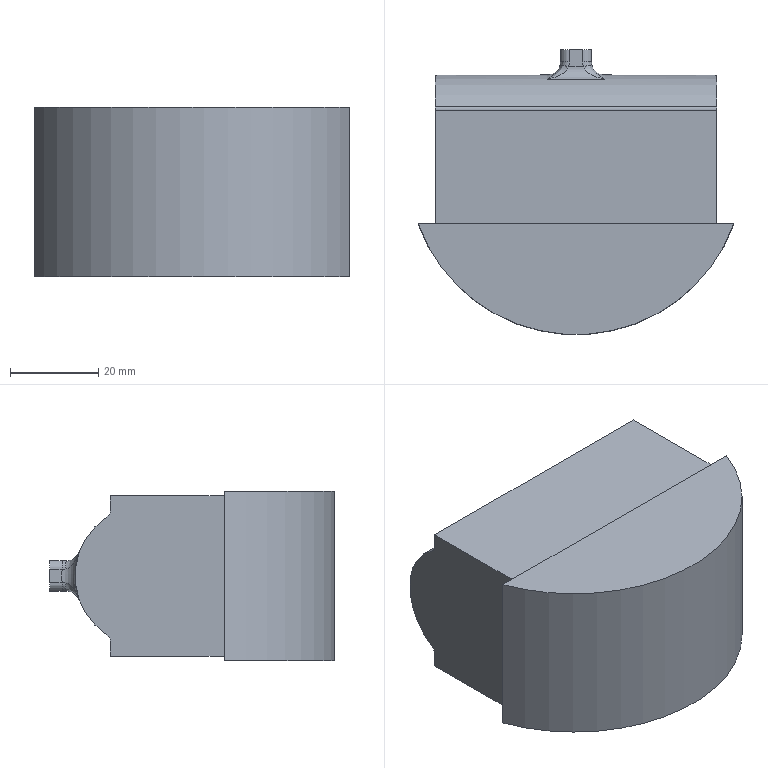Part | 1 solid | 34 faces | box 71.627 x 64.667 x 38.42 mm | volume 120668 mm3 | plane 14 | cylinder 10 | spline 8 | torus 2 | commonest cylinder face diameters 4 x4 3.6 x2 6 x2 32 x1 76.2 x1
STEP:
#1=CARTESIAN_POINT('',(-35.814,-13.,19.21));
#2=VERTEX_POINT('',#1);
#3=CARTESIAN_POINT('',(35.814,-13.,19.21));
#4=VERTEX_POINT('',#3);
#5=CARTESIAN_POINT('',(0.,0.,19.21));
#6=DIRECTION('',(0.,0.,1.));
#7=DIRECTION('',(1.,0.,0.));
#8=AXIS2_PLACEMENT_3D('',#5,#6,#7);
#9=CIRCLE('',#8,38.1);
#10=EDGE_CURVE('',#2,#4,#9,.T.);
#11=ORIENTED_EDGE('',*,*,#10,.F.);
#12=CARTESIAN_POINT('',(-35.814,-13.,-19.21));
#13=VERTEX_POINT('',#12);
#14=CARTESIAN_POINT('',(-35.814,-13.,-19.21));
#15=DIRECTION('',(0.,0.,1.));
#16=VECTOR('',#15,1000.);
#17=LINE('',#14,#16);
#18=EDGE_CURVE('',#2,#13,#17,.F.);
#19=ORIENTED_EDGE('',*,*,#18,.T.);
#20=CARTESIAN_POINT('',(35.814,-13.,-19.21));
#21=VERTEX_POINT('',#20);
#22=CARTESIAN_POINT('',(0.,0.,-19.21));
#23=DIRECTION('',(0.,0.,1.));
#24=DIRECTION('',(1.,0.,0.));
#25=AXIS2_PLACEMENT_3D('',#22,#23,#24);
#26=CIRCLE('',#25,38.1);
#27=EDGE_CURVE('',#13,#21,#26,.T.);
#28=ORIENTED_EDGE('',*,*,#27,.T.);
#29=CARTESIAN_POINT('',(35.814,-13.,-19.21));
#30=DIRECTION('',(0.,0.,1.));
#31=VECTOR('',#30,1000.);
#32=LINE('',#29,#31);
#33=EDGE_CURVE('',#21,#4,#32,.T.);
#34=ORIENTED_EDGE('',*,*,#33,.T.);
#35=EDGE_LOOP('',(#11,#19,#28,#34));
#36=FACE_BOUND('',#35,.T.);
#37=CARTESIAN_POINT('',(0.,0.,-19.21));
#38=DIRECTION('',(0.,0.,1.));
#39=DIRECTION('',(1.,0.,0.));
#40=AXIS2_PLACEMENT_3D('',#37,#38,#39);
#41=CYLINDRICAL_SURFACE('',#40,38.1);
#42=ADVANCED_FACE('',(#36),#41,.T.);
#43=CARTESIAN_POINT('',(0.,-13.,-19.21));
#44=DIRECTION('',(-1.,0.,0.));
#45=VECTOR('',#44,1000.);
#46=LINE('',#43,#45);
#47=EDGE_CURVE('',#21,#13,#46,.T.);
#48=ORIENTED_EDGE('',*,*,#47,.F.);
#49=ORIENTED_EDGE('',*,*,#27,.F.);
#50=EDGE_LOOP('',(#48,#49));
#51=FACE_BOUND('',#50,.T.);
#52=CARTESIAN_POINT('',(0.,0.,-19.21));
#53=DIRECTION('',(0.,0.,1.));
#54=DIRECTION('',(1.,0.,0.));
#55=AXIS2_PLACEMENT_3D('',#52,#53,#54);
#56=PLANE('',#55);
#57=ADVANCED_FACE('',(#51),#56,.F.);
#58=ORIENTED_EDGE('',*,*,#10,.T.);
#59=CARTESIAN_POINT('',(0.,-13.,19.21));
#60=DIRECTION('',(-1.,0.,0.));
#61=VECTOR('',#60,1000.);
#62=LINE('',#59,#61);
#63=EDGE_CURVE('',#4,#2,#62,.T.);
#64=ORIENTED_EDGE('',*,*,#63,.T.);
#65=EDGE_LOOP('',(#58,#64));
#66=FACE_BOUND('',#65,.T.);
#67=CARTESIAN_POINT('',(0.,0.,19.21));
#68=DIRECTION('',(0.,0.,1.));
#69=DIRECTION('',(1.,0.,0.));
#70=AXIS2_PLACEMENT_3D('',#67,#68,#69);
#71=PLANE('',#70);
#72=ADVANCED_FACE('',(#66),#71,.T.);
#73=CARTESIAN_POINT('',(31.91,-13.,18.207));
#74=VERTEX_POINT('',#73);
#75=CARTESIAN_POINT('',(31.91,-13.,-18.207));
#76=VERTEX_POINT('',#75);
#77=CARTESIAN_POINT('',(31.91,-13.,18.207));
#78=DIRECTION('',(0.,0.,-1.));
#79=VECTOR('',#78,1000.);
#80=LINE('',#77,#79);
#81=EDGE_CURVE('',#74,#76,#80,.T.);
#82=ORIENTED_EDGE('',*,*,#81,.F.);
#83=CARTESIAN_POINT('',(-31.91,-13.,18.207));
#84=VERTEX_POINT('',#83);
#85=CARTESIAN_POINT('',(-31.91,-13.,18.207));
#86=DIRECTION('',(1.,0.,0.));
#87=VECTOR('',#86,1000.);
#88=LINE('',#85,#87);
#89=EDGE_CURVE('',#84,#74,#88,.T.);
#90=ORIENTED_EDGE('',*,*,#89,.F.);
#91=CARTESIAN_POINT('',(-31.91,-13.,-18.207));
#92=VERTEX_POINT('',#91);
#93=CARTESIAN_POINT('',(-31.91,-13.,18.207));
#94=DIRECTION('',(0.,0.,1.));
#95=VECTOR('',#94,1000.);
#96=LINE('',#93,#95);
#97=EDGE_CURVE('',#92,#84,#96,.T.);
#98=ORIENTED_EDGE('',*,*,#97,.F.);
#99=CARTESIAN_POINT('',(-31.91,-13.,-18.207));
#100=DIRECTION('',(-1.,0.,0.));
#101=VECTOR('',#100,1000.);
#102=LINE('',#99,#101);
#103=EDGE_CURVE('',#76,#92,#102,.T.);
#104=ORIENTED_EDGE('',*,*,#103,.F.);
#105=EDGE_LOOP('',(#82,#90,#98,#104));
#106=FACE_BOUND('',#105,.T.);
#107=ORIENTED_EDGE('',*,*,#47,.T.);
#108=ORIENTED_EDGE('',*,*,#18,.F.);
#109=ORIENTED_EDGE('',*,*,#63,.F.);
#110=ORIENTED_EDGE('',*,*,#33,.F.);
#111=EDGE_LOOP('',(#107,#108,#109,#110));
#112=FACE_BOUND('',#111,.T.);
#113=CARTESIAN_POINT('',(0.,-13.,0.));
#114=DIRECTION('',(0.,1.,0.));
#115=DIRECTION('',(0.,0.,1.));
#116=AXIS2_PLACEMENT_3D('',#113,#114,#115);
#117=PLANE('',#116);
#118=ADVANCED_FACE('',(#106,#112),#117,.T.);
#119=CARTESIAN_POINT('',(31.91,12.817,-18.207));
#120=VERTEX_POINT('',#119);
#121=CARTESIAN_POINT('',(-31.91,12.817,-18.207));
#122=VERTEX_POINT('',#121);
#123=CARTESIAN_POINT('',(-31.91,12.817,-18.207));
#124=DIRECTION('',(-1.,0.,0.));
#125=VECTOR('',#124,1000.);
#126=LINE('',#123,#125);
#127=EDGE_CURVE('',#120,#122,#126,.T.);
#128=ORIENTED_EDGE('',*,*,#127,.F.);
#129=CARTESIAN_POINT('',(31.91,-13.,-18.207));
#130=DIRECTION('',(0.,1.,0.));
#131=VECTOR('',#130,1000.);
#132=LINE('',#129,#131);
#133=EDGE_CURVE('',#76,#120,#132,.T.);
#134=ORIENTED_EDGE('',*,*,#133,.F.);
#135=ORIENTED_EDGE('',*,*,#103,.T.);
#136=CARTESIAN_POINT('',(-31.91,-13.,-18.207));
#137=DIRECTION('',(0.,1.,0.));
#138=VECTOR('',#137,1000.);
#139=LINE('',#136,#138);
#140=EDGE_CURVE('',#92,#122,#139,.T.);
#141=ORIENTED_EDGE('',*,*,#140,.T.);
#142=EDGE_LOOP('',(#128,#134,#135,#141));
#143=FACE_BOUND('',#142,.T.);
#144=CARTESIAN_POINT('',(-31.91,-13.,-18.207));
#145=DIRECTION('',(0.,0.,-1.));
#146=DIRECTION('',(-1.,0.,0.));
#147=AXIS2_PLACEMENT_3D('',#144,#145,#146);
#148=PLANE('',#147);
#149=ADVANCED_FACE('',(#143),#148,.T.);
#150=CARTESIAN_POINT('',(31.91,12.817,-14.859));
#151=VERTEX_POINT('',#150);
#152=CARTESIAN_POINT('',(31.91,12.817,-13.856));
#153=DIRECTION('',(0.,0.,-1.));
#154=VECTOR('',#153,1000.);
#155=LINE('',#152,#154);
#156=EDGE_CURVE('',#151,#120,#155,.T.);
#157=ORIENTED_EDGE('',*,*,#156,.F.);
#158=CARTESIAN_POINT('',(31.91,13.626,-13.357));
#159=VERTEX_POINT('',#158);
#160=CARTESIAN_POINT('',(31.91,14.617,-14.859));
#161=DIRECTION('',(1.,0.,0.));
#162=DIRECTION('',(0.,0.,-1.));
#163=AXIS2_PLACEMENT_3D('',#160,#161,#162);
#164=CIRCLE('',#163,1.8);
#165=EDGE_CURVE('',#151,#159,#164,.F.);
#166=ORIENTED_EDGE('',*,*,#165,.T.);
#167=CARTESIAN_POINT('',(31.91,13.626,13.357));
#168=VERTEX_POINT('',#167);
#169=CARTESIAN_POINT('',(31.91,4.817,0.));
#170=DIRECTION('',(-1.,0.,0.));
#171=DIRECTION('',(0.,0.,-1.));
#172=AXIS2_PLACEMENT_3D('',#169,#170,#171);
#173=CIRCLE('',#172,16.);
#174=EDGE_CURVE('',#168,#159,#173,.T.);
#175=ORIENTED_EDGE('',*,*,#174,.F.);
#176=CARTESIAN_POINT('',(31.91,12.817,14.859));
#177=VERTEX_POINT('',#176);
#178=CARTESIAN_POINT('',(31.91,14.617,14.859));
#179=DIRECTION('',(1.,0.,0.));
#180=DIRECTION('',(0.,0.,-1.));
#181=AXIS2_PLACEMENT_3D('',#178,#179,#180);
#182=CIRCLE('',#181,1.8);
#183=EDGE_CURVE('',#168,#177,#182,.F.);
#184=ORIENTED_EDGE('',*,*,#183,.T.);
#185=CARTESIAN_POINT('',(31.91,12.817,18.207));
#186=VERTEX_POINT('',#185);
#187=CARTESIAN_POINT('',(31.91,12.817,20.785));
#188=DIRECTION('',(0.,0.,-1.));
#189=VECTOR('',#188,1000.);
#190=LINE('',#187,#189);
#191=EDGE_CURVE('',#186,#177,#190,.T.);
#192=ORIENTED_EDGE('',*,*,#191,.F.);
#193=CARTESIAN_POINT('',(31.91,-13.,18.207));
#194=DIRECTION('',(0.,1.,0.));
#195=VECTOR('',#194,1000.);
#196=LINE('',#193,#195);
#197=EDGE_CURVE('',#74,#186,#196,.T.);
#198=ORIENTED_EDGE('',*,*,#197,.F.);
#199=ORIENTED_EDGE('',*,*,#81,.T.);
#200=ORIENTED_EDGE('',*,*,#133,.T.);
#201=EDGE_LOOP('',(#157,#166,#175,#184,#192,#198,#199,#200));
#202=FACE_BOUND('',#201,.T.);
#203=CARTESIAN_POINT('',(31.91,-13.,18.207));
#204=DIRECTION('',(1.,0.,0.));
#205=DIRECTION('',(0.,0.,-1.));
#206=AXIS2_PLACEMENT_3D('',#203,#204,#205);
#207=PLANE('',#206);
#208=ADVANCED_FACE('',(#202),#207,.T.);
#209=CARTESIAN_POINT('',(-31.91,12.817,18.207));
#210=VERTEX_POINT('',#209);
#211=CARTESIAN_POINT('',(-31.91,12.817,18.207));
#212=DIRECTION('',(1.,0.,0.));
#213=VECTOR('',#212,1000.);
#214=LINE('',#211,#213);
#215=EDGE_CURVE('',#210,#186,#214,.T.);
#216=ORIENTED_EDGE('',*,*,#215,.F.);
#217=CARTESIAN_POINT('',(-31.91,-13.,18.207));
#218=DIRECTION('',(0.,1.,0.));
#219=VECTOR('',#218,1000.);
#220=LINE('',#217,#219);
#221=EDGE_CURVE('',#84,#210,#220,.T.);
#222=ORIENTED_EDGE('',*,*,#221,.F.);
#223=ORIENTED_EDGE('',*,*,#89,.T.);
#224=ORIENTED_EDGE('',*,*,#197,.T.);
#225=EDGE_LOOP('',(#216,#222,#223,#224));
#226=FACE_BOUND('',#225,.T.);
#227=CARTESIAN_POINT('',(-31.91,-13.,18.207));
#228=DIRECTION('',(0.,0.,1.));
#229=DIRECTION('',(1.,0.,0.));
#230=AXIS2_PLACEMENT_3D('',#227,#228,#229);
#231=PLANE('',#230);
#232=ADVANCED_FACE('',(#226),#231,.T.);
#233=CARTESIAN_POINT('',(-31.91,12.817,-14.859));
#234=VERTEX_POINT('',#233);
#235=CARTESIAN_POINT('',(-31.91,12.817,18.207));
#236=DIRECTION('',(0.,0.,1.));
#237=VECTOR('',#236,1000.);
#238=LINE('',#235,#237);
#239=EDGE_CURVE('',#122,#234,#238,.T.);
#240=ORIENTED_EDGE('',*,*,#239,.F.);
#241=ORIENTED_EDGE('',*,*,#140,.F.);
#242=ORIENTED_EDGE('',*,*,#97,.T.);
#243=ORIENTED_EDGE('',*,*,#221,.T.);
#244=CARTESIAN_POINT('',(-31.91,12.817,14.859));
#245=VERTEX_POINT('',#244);
#246=CARTESIAN_POINT('',(-31.91,12.817,18.207));
#247=DIRECTION('',(0.,0.,1.));
#248=VECTOR('',#247,1000.);
#249=LINE('',#246,#248);
#250=EDGE_CURVE('',#245,#210,#249,.T.);
#251=ORIENTED_EDGE('',*,*,#250,.F.);
#252=CARTESIAN_POINT('',(-31.91,13.626,13.357));
#253=VERTEX_POINT('',#252);
#254=CARTESIAN_POINT('',(-31.91,14.617,14.859));
#255=DIRECTION('',(-1.,0.,0.));
#256=DIRECTION('',(0.,0.,1.));
#257=AXIS2_PLACEMENT_3D('',#254,#255,#256);
#258=CIRCLE('',#257,1.8);
#259=EDGE_CURVE('',#245,#253,#258,.F.);
#260=ORIENTED_EDGE('',*,*,#259,.T.);
#261=CARTESIAN_POINT('',(-31.91,13.626,-13.357));
#262=VERTEX_POINT('',#261);
#263=CARTESIAN_POINT('',(-31.91,4.817,0.));
#264=DIRECTION('',(-1.,0.,0.));
#265=DIRECTION('',(0.,0.,1.));
#266=AXIS2_PLACEMENT_3D('',#263,#264,#265);
#267=CIRCLE('',#266,16.);
#268=EDGE_CURVE('',#262,#253,#267,.F.);
#269=ORIENTED_EDGE('',*,*,#268,.F.);
#270=CARTESIAN_POINT('',(-31.91,14.617,-14.859));
#271=DIRECTION('',(-1.,0.,0.));
#272=DIRECTION('',(0.,0.,1.));
#273=AXIS2_PLACEMENT_3D('',#270,#271,#272);
#274=CIRCLE('',#273,1.8);
#275=EDGE_CURVE('',#262,#234,#274,.F.);
#276=ORIENTED_EDGE('',*,*,#275,.T.);
#277=EDGE_LOOP('',(#240,#241,#242,#243,#251,#260,#269,#276));
#278=FACE_BOUND('',#277,.T.);
#279=CARTESIAN_POINT('',(-31.91,-13.,18.207));
#280=DIRECTION('',(-1.,0.,0.));
#281=DIRECTION('',(0.,0.,1.));
#282=AXIS2_PLACEMENT_3D('',#279,#280,#281);
#283=PLANE('',#282);
#284=ADVANCED_FACE('',(#278),#283,.T.);
#285=CARTESIAN_POINT('',(6.5,19.852,-5.474));
#286=VERTEX_POINT('',#285);
#287=CARTESIAN_POINT('',(6.5,19.852,5.474));
#288=VERTEX_POINT('',#287);
#289=CARTESIAN_POINT('',(6.5,4.817,0.));
#290=DIRECTION('',(1.,0.,0.));
#291=DIRECTION('',(0.,0.,-1.));
#292=AXIS2_PLACEMENT_3D('',#289,#290,#291);
#293=CIRCLE('',#292,16.);
#294=EDGE_CURVE('',#286,#288,#293,.T.);
#295=ORIENTED_EDGE('',*,*,#294,.T.);
#296=CARTESIAN_POINT('',(-6.5,19.852,5.474));
#297=VERTEX_POINT('',#296);
#298=CARTESIAN_POINT('',(-35.814,19.852,5.474));
#299=DIRECTION('',(1.,0.,0.));
#300=VECTOR('',#299,1000.);
#301=LINE('',#298,#300);
#302=EDGE_CURVE('',#288,#297,#301,.F.);
#303=ORIENTED_EDGE('',*,*,#302,.T.);
#304=CARTESIAN_POINT('',(-6.5,19.852,-5.474));
#305=VERTEX_POINT('',#304);
#306=CARTESIAN_POINT('',(-6.5,4.817,0.));
#307=DIRECTION('',(-1.,0.,0.));
#308=DIRECTION('',(0.,0.,1.));
#309=AXIS2_PLACEMENT_3D('',#306,#307,#308);
#310=CIRCLE('',#309,16.);
#311=EDGE_CURVE('',#297,#305,#310,.T.);
#312=ORIENTED_EDGE('',*,*,#311,.T.);
#313=CARTESIAN_POINT('',(-35.814,19.852,-5.474));
#314=DIRECTION('',(1.,0.,0.));
#315=VECTOR('',#314,1000.);
#316=LINE('',#313,#315);
#317=EDGE_CURVE('',#305,#286,#316,.T.);
#318=ORIENTED_EDGE('',*,*,#317,.T.);
#319=EDGE_LOOP('',(#295,#303,#312,#318));
#320=FACE_BOUND('',#319,.T.);
#321=ORIENTED_EDGE('',*,*,#268,.T.);
#322=CARTESIAN_POINT('',(-35.814,13.626,13.357));
#323=DIRECTION('',(1.,0.,0.));
#324=VECTOR('',#323,1000.);
#325=LINE('',#322,#324);
#326=EDGE_CURVE('',#253,#168,#325,.T.);
#327=ORIENTED_EDGE('',*,*,#326,.T.);
#328=ORIENTED_EDGE('',*,*,#174,.T.);
#329=CARTESIAN_POINT('',(-35.814,13.626,-13.357));
#330=DIRECTION('',(1.,0.,0.));
#331=VECTOR('',#330,1000.);
#332=LINE('',#329,#331);
#333=EDGE_CURVE('',#159,#262,#332,.F.);
#334=ORIENTED_EDGE('',*,*,#333,.T.);
#335=EDGE_LOOP('',(#321,#327,#328,#334));
#336=FACE_BOUND('',#335,.T.);
#337=CARTESIAN_POINT('',(-35.814,4.817,0.));
#338=DIRECTION('',(1.,0.,0.));
#339=DIRECTION('',(0.,0.,-1.));
#340=AXIS2_PLACEMENT_3D('',#337,#338,#339);
#341=CYLINDRICAL_SURFACE('',#340,16.);
#342=ADVANCED_FACE('',(#320,#336),#341,.T.);
#343=ORIENTED_EDGE('',*,*,#239,.T.);
#344=CARTESIAN_POINT('',(31.91,12.817,-14.859));
#345=DIRECTION('',(-1.,0.,0.));
#346=VECTOR('',#345,1000.);
#347=LINE('',#344,#346);
#348=EDGE_CURVE('',#234,#151,#347,.F.);
#349=ORIENTED_EDGE('',*,*,#348,.T.);
#350=ORIENTED_EDGE('',*,*,#156,.T.);
#351=ORIENTED_EDGE('',*,*,#127,.T.);
#352=EDGE_LOOP('',(#343,#349,#350,#351));
#353=FACE_BOUND('',#352,.T.);
#354=CARTESIAN_POINT('',(-35.814,12.817,-13.856));
#355=DIRECTION('',(0.,-1.,0.));
#356=DIRECTION('',(0.,0.,-1.));
#357=AXIS2_PLACEMENT_3D('',#354,#355,#356);
#358=PLANE('',#357);
#359=ADVANCED_FACE('',(#353),#358,.F.);
#360=ORIENTED_EDGE('',*,*,#191,.T.);
#361=CARTESIAN_POINT('',(-31.91,12.817,14.859));
#362=DIRECTION('',(-1.,0.,0.));
#363=VECTOR('',#362,1000.);
#364=LINE('',#361,#363);
#365=EDGE_CURVE('',#177,#245,#364,.T.);
#366=ORIENTED_EDGE('',*,*,#365,.T.);
#367=ORIENTED_EDGE('',*,*,#250,.T.);
#368=ORIENTED_EDGE('',*,*,#215,.T.);
#369=EDGE_LOOP('',(#360,#366,#367,#368));
#370=FACE_BOUND('',#369,.T.);
#371=CARTESIAN_POINT('',(-35.814,12.817,20.785));
#372=DIRECTION('',(0.,-1.,0.));
#373=DIRECTION('',(0.,0.,-1.));
#374=AXIS2_PLACEMENT_3D('',#371,#372,#373);
#375=PLANE('',#374);
#376=ADVANCED_FACE('',(#370),#375,.F.);
#377=ORIENTED_EDGE('',*,*,#259,.F.);
#378=ORIENTED_EDGE('',*,*,#365,.F.);
#379=ORIENTED_EDGE('',*,*,#183,.F.);
#380=ORIENTED_EDGE('',*,*,#326,.F.);
#381=EDGE_LOOP('',(#377,#378,#379,#380));
#382=FACE_BOUND('',#381,.T.);
#383=CARTESIAN_POINT('',(-35.814,14.617,14.859));
#384=DIRECTION('',(1.,0.,0.));
#385=DIRECTION('',(0.,0.,-1.));
#386=AXIS2_PLACEMENT_3D('',#383,#384,#385);
#387=CYLINDRICAL_SURFACE('',#386,1.8);
#388=ADVANCED_FACE('',(#382),#387,.F.);
#389=ORIENTED_EDGE('',*,*,#275,.F.);
#390=ORIENTED_EDGE('',*,*,#333,.F.);
#391=ORIENTED_EDGE('',*,*,#165,.F.);
#392=ORIENTED_EDGE('',*,*,#348,.F.);
#393=EDGE_LOOP('',(#389,#390,#391,#392));
#394=FACE_BOUND('',#393,.T.);
#395=CARTESIAN_POINT('',(-35.814,14.617,-14.859));
#396=DIRECTION('',(1.,0.,0.));
#397=DIRECTION('',(0.,0.,-1.));
#398=AXIS2_PLACEMENT_3D('',#395,#396,#397);
#399=CYLINDRICAL_SURFACE('',#398,1.8);
#400=ADVANCED_FACE('',(#394),#399,.F.);
#401=CARTESIAN_POINT('',(3.5,23.758,1.5));
#402=VERTEX_POINT('',#401);
#403=CARTESIAN_POINT('',(3.5,23.758,-1.5));
#404=VERTEX_POINT('',#403);
#405=CARTESIAN_POINT('',(3.5,4.817,0.));
#406=DIRECTION('',(1.,0.,0.));
#407=DIRECTION('',(0.,0.,-1.));
#408=AXIS2_PLACEMENT_3D('',#405,#406,#407);
#409=CIRCLE('',#408,19.);
#410=EDGE_CURVE('',#402,#404,#409,.F.);
#411=ORIENTED_EDGE('',*,*,#410,.T.);
#412=CARTESIAN_POINT('',(3.5,26.567,-1.5));
#413=VERTEX_POINT('',#412);
#414=CARTESIAN_POINT('',(3.5,16.924,-1.5));
#415=DIRECTION('',(0.,1.,0.));
#416=VECTOR('',#415,1000.);
#417=LINE('',#414,#416);
#418=EDGE_CURVE('',#404,#413,#417,.T.);
#419=ORIENTED_EDGE('',*,*,#418,.T.);
#420=CARTESIAN_POINT('',(3.5,26.567,1.5));
#421=VERTEX_POINT('',#420);
#422=CARTESIAN_POINT('',(3.5,26.567,-3.5));
#423=DIRECTION('',(0.,0.,-1.));
#424=VECTOR('',#423,1000.);
#425=LINE('',#422,#424);
#426=EDGE_CURVE('',#421,#413,#425,.T.);
#427=ORIENTED_EDGE('',*,*,#426,.F.);
#428=CARTESIAN_POINT('',(3.5,16.924,1.5));
#429=DIRECTION('',(0.,1.,0.));
#430=VECTOR('',#429,1000.);
#431=LINE('',#428,#430);
#432=EDGE_CURVE('',#421,#402,#431,.F.);
#433=ORIENTED_EDGE('',*,*,#432,.T.);
#434=EDGE_LOOP('',(#411,#419,#427,#433));
#435=FACE_BOUND('',#434,.T.);
#436=CARTESIAN_POINT('',(3.5,16.924,-3.5));
#437=DIRECTION('',(1.,0.,0.));
#438=DIRECTION('',(0.,0.,-1.));
#439=AXIS2_PLACEMENT_3D('',#436,#437,#438);
#440=PLANE('',#439);
#441=ADVANCED_FACE('',(#435),#440,.T.);
#442=CARTESIAN_POINT('',(-1.619,22.671,3.5));
#443=VERTEX_POINT('',#442);
#444=CARTESIAN_POINT('',(1.619,22.671,3.5));
#445=VERTEX_POINT('',#444);
#446=CARTESIAN_POINT('',(-3.5,22.671,3.5));
#447=DIRECTION('',(1.,0.,0.));
#448=VECTOR('',#447,1000.);
#449=LINE('',#446,#448);
#450=EDGE_CURVE('',#443,#445,#449,.T.);
#451=ORIENTED_EDGE('',*,*,#450,.T.);
#452=CARTESIAN_POINT('',(1.5,23.758,3.5));
#453=VERTEX_POINT('',#452);
#454=CARTESIAN_POINT('',(1.619,22.671,3.5));
#455=CARTESIAN_POINT('',(1.54,23.029,3.5));
#456=CARTESIAN_POINT('',(1.5,23.391,3.5));
#457=CARTESIAN_POINT('',(1.5,23.758,3.5));
#458=B_SPLINE_CURVE_WITH_KNOTS('',3,(#454,#455,#456,#457),.UNSPECIFIED.,.F.,.F.,(4,4),(0.,0.001094),.UNSPECIFIED.);
#459=EDGE_CURVE('',#445,#453,#458,.T.);
#460=ORIENTED_EDGE('',*,*,#459,.T.);
#461=CARTESIAN_POINT('',(1.5,26.567,3.5));
#462=VERTEX_POINT('',#461);
#463=CARTESIAN_POINT('',(1.5,16.924,3.5));
#464=DIRECTION('',(0.,1.,0.));
#465=VECTOR('',#464,1000.);
#466=LINE('',#463,#465);
#467=EDGE_CURVE('',#453,#462,#466,.T.);
#468=ORIENTED_EDGE('',*,*,#467,.T.);
#469=CARTESIAN_POINT('',(-1.5,26.567,3.5));
#470=VERTEX_POINT('',#469);
#471=CARTESIAN_POINT('',(-3.5,26.567,3.5));
#472=DIRECTION('',(1.,0.,0.));
#473=VECTOR('',#472,1000.);
#474=LINE('',#471,#473);
#475=EDGE_CURVE('',#470,#462,#474,.T.);
#476=ORIENTED_EDGE('',*,*,#475,.F.);
#477=CARTESIAN_POINT('',(-1.5,23.758,3.5));
#478=VERTEX_POINT('',#477);
#479=CARTESIAN_POINT('',(-1.5,16.924,3.5));
#480=DIRECTION('',(0.,1.,0.));
#481=VECTOR('',#480,1000.);
#482=LINE('',#479,#481);
#483=EDGE_CURVE('',#470,#478,#482,.F.);
#484=ORIENTED_EDGE('',*,*,#483,.T.);
#485=CARTESIAN_POINT('',(-1.5,23.758,3.5));
#486=CARTESIAN_POINT('',(-1.5,23.391,3.5));
#487=CARTESIAN_POINT('',(-1.54,23.029,3.5));
#488=CARTESIAN_POINT('',(-1.619,22.671,3.5));
#489=B_SPLINE_CURVE_WITH_KNOTS('',3,(#485,#486,#487,#488),.UNSPECIFIED.,.F.,.F.,(4,4),(0.,0.001094),.UNSPECIFIED.);
#490=EDGE_CURVE('',#478,#443,#489,.T.);
#491=ORIENTED_EDGE('',*,*,#490,.T.);
#492=EDGE_LOOP('',(#451,#460,#468,#476,#484,#491));
#493=FACE_BOUND('',#492,.T.);
#494=CARTESIAN_POINT('',(-3.5,16.924,3.5));
#495=DIRECTION('',(0.,0.,1.));
#496=DIRECTION('',(1.,0.,0.));
#497=AXIS2_PLACEMENT_3D('',#494,#495,#496);
#498=PLANE('',#497);
#499=ADVANCED_FACE('',(#493),#498,.T.);
#500=CARTESIAN_POINT('',(-3.5,26.567,-1.5));
#501=VERTEX_POINT('',#500);
#502=CARTESIAN_POINT('',(-3.5,26.567,1.5));
#503=VERTEX_POINT('',#502);
#504=CARTESIAN_POINT('',(-3.5,26.567,-3.5));
#505=DIRECTION('',(0.,0.,1.));
#506=VECTOR('',#505,1000.);
#507=LINE('',#504,#506);
#508=EDGE_CURVE('',#501,#503,#507,.T.);
#509=ORIENTED_EDGE('',*,*,#508,.F.);
#510=CARTESIAN_POINT('',(-3.5,23.758,-1.5));
#511=VERTEX_POINT('',#510);
#512=CARTESIAN_POINT('',(-3.5,16.924,-1.5));
#513=DIRECTION('',(0.,1.,0.));
#514=VECTOR('',#513,1000.);
#515=LINE('',#512,#514);
#516=EDGE_CURVE('',#501,#511,#515,.F.);
#517=ORIENTED_EDGE('',*,*,#516,.T.);
#518=CARTESIAN_POINT('',(-3.5,23.758,1.5));
#519=VERTEX_POINT('',#518);
#520=CARTESIAN_POINT('',(-3.5,4.817,0.));
#521=DIRECTION('',(-1.,0.,0.));
#522=DIRECTION('',(0.,0.,1.));
#523=AXIS2_PLACEMENT_3D('',#520,#521,#522);
#524=CIRCLE('',#523,19.);
#525=EDGE_CURVE('',#511,#519,#524,.F.);
#526=ORIENTED_EDGE('',*,*,#525,.T.);
#527=CARTESIAN_POINT('',(-3.5,16.924,1.5));
#528=DIRECTION('',(0.,1.,0.));
#529=VECTOR('',#528,1000.);
#530=LINE('',#527,#529);
#531=EDGE_CURVE('',#519,#503,#530,.T.);
#532=ORIENTED_EDGE('',*,*,#531,.T.);
#533=EDGE_LOOP('',(#509,#517,#526,#532));
#534=FACE_BOUND('',#533,.T.);
#535=CARTESIAN_POINT('',(-3.5,16.924,-3.5));
#536=DIRECTION('',(-1.,0.,0.));
#537=DIRECTION('',(0.,0.,1.));
#538=AXIS2_PLACEMENT_3D('',#535,#536,#537);
#539=PLANE('',#538);
#540=ADVANCED_FACE('',(#534),#539,.T.);
#541=CARTESIAN_POINT('',(1.619,22.671,-3.5));
#542=VERTEX_POINT('',#541);
#543=CARTESIAN_POINT('',(-1.619,22.671,-3.5));
#544=VERTEX_POINT('',#543);
#545=CARTESIAN_POINT('',(-3.5,22.671,-3.5));
#546=DIRECTION('',(1.,0.,0.));
#547=VECTOR('',#546,1000.);
#548=LINE('',#545,#547);
#549=EDGE_CURVE('',#542,#544,#548,.F.);
#550=ORIENTED_EDGE('',*,*,#549,.T.);
#551=CARTESIAN_POINT('',(-1.5,23.758,-3.5));
#552=VERTEX_POINT('',#551);
#553=CARTESIAN_POINT('',(-1.619,22.671,-3.5));
#554=CARTESIAN_POINT('',(-1.54,23.029,-3.5));
#555=CARTESIAN_POINT('',(-1.5,23.391,-3.5));
#556=CARTESIAN_POINT('',(-1.5,23.758,-3.5));
#557=B_SPLINE_CURVE_WITH_KNOTS('',3,(#553,#554,#555,#556),.UNSPECIFIED.,.F.,.F.,(4,4),(0.,0.001094),.UNSPECIFIED.);
#558=EDGE_CURVE('',#544,#552,#557,.T.);
#559=ORIENTED_EDGE('',*,*,#558,.T.);
#560=CARTESIAN_POINT('',(-1.5,26.567,-3.5));
#561=VERTEX_POINT('',#560);
#562=CARTESIAN_POINT('',(-1.5,16.924,-3.5));
#563=DIRECTION('',(0.,1.,0.));
#564=VECTOR('',#563,1000.);
#565=LINE('',#562,#564);
#566=EDGE_CURVE('',#552,#561,#565,.T.);
#567=ORIENTED_EDGE('',*,*,#566,.T.);
#568=CARTESIAN_POINT('',(1.5,26.567,-3.5));
#569=VERTEX_POINT('',#568);
#570=CARTESIAN_POINT('',(-3.5,26.567,-3.5));
#571=DIRECTION('',(-1.,0.,0.));
#572=VECTOR('',#571,1000.);
#573=LINE('',#570,#572);
#574=EDGE_CURVE('',#569,#561,#573,.T.);
#575=ORIENTED_EDGE('',*,*,#574,.F.);
#576=CARTESIAN_POINT('',(1.5,23.758,-3.5));
#577=VERTEX_POINT('',#576);
#578=CARTESIAN_POINT('',(1.5,16.924,-3.5));
#579=DIRECTION('',(0.,1.,0.));
#580=VECTOR('',#579,1000.);
#581=LINE('',#578,#580);
#582=EDGE_CURVE('',#569,#577,#581,.F.);
#583=ORIENTED_EDGE('',*,*,#582,.T.);
#584=CARTESIAN_POINT('',(1.5,23.758,-3.5));
#585=CARTESIAN_POINT('',(1.5,23.391,-3.5));
#586=CARTESIAN_POINT('',(1.54,23.029,-3.5));
#587=CARTESIAN_POINT('',(1.619,22.671,-3.5));
#588=B_SPLINE_CURVE_WITH_KNOTS('',3,(#584,#585,#586,#587),.UNSPECIFIED.,.F.,.F.,(4,4),(0.,0.001094),.UNSPECIFIED.);
#589=EDGE_CURVE('',#577,#542,#588,.T.);
#590=ORIENTED_EDGE('',*,*,#589,.T.);
#591=EDGE_LOOP('',(#550,#559,#567,#575,#583,#590));
#592=FACE_BOUND('',#591,.T.);
#593=CARTESIAN_POINT('',(-3.5,16.924,-3.5));
#594=DIRECTION('',(0.,0.,-1.));
#595=DIRECTION('',(-1.,0.,0.));
#596=AXIS2_PLACEMENT_3D('',#593,#594,#595);
#597=PLANE('',#596);
#598=ADVANCED_FACE('',(#592),#597,.T.);
#599=ORIENTED_EDGE('',*,*,#574,.T.);
#600=CARTESIAN_POINT('',(-1.5,26.567,-1.5));
#601=DIRECTION('',(0.,1.,0.));
#602=DIRECTION('',(0.,0.,1.));
#603=AXIS2_PLACEMENT_3D('',#600,#601,#602);
#604=CIRCLE('',#603,2.);
#605=EDGE_CURVE('',#561,#501,#604,.T.);
#606=ORIENTED_EDGE('',*,*,#605,.T.);
#607=ORIENTED_EDGE('',*,*,#508,.T.);
#608=CARTESIAN_POINT('',(-1.5,26.567,1.5));
#609=DIRECTION('',(0.,1.,0.));
#610=DIRECTION('',(0.,0.,1.));
#611=AXIS2_PLACEMENT_3D('',#608,#609,#610);
#612=CIRCLE('',#611,2.);
#613=EDGE_CURVE('',#503,#470,#612,.T.);
#614=ORIENTED_EDGE('',*,*,#613,.T.);
#615=ORIENTED_EDGE('',*,*,#475,.T.);
#616=CARTESIAN_POINT('',(1.5,26.567,1.5));
#617=DIRECTION('',(0.,1.,0.));
#618=DIRECTION('',(0.,0.,1.));
#619=AXIS2_PLACEMENT_3D('',#616,#617,#618);
#620=CIRCLE('',#619,2.);
#621=EDGE_CURVE('',#462,#421,#620,.T.);
#622=ORIENTED_EDGE('',*,*,#621,.T.);
#623=ORIENTED_EDGE('',*,*,#426,.T.);
#624=CARTESIAN_POINT('',(1.5,26.567,-1.5));
#625=DIRECTION('',(0.,1.,0.));
#626=DIRECTION('',(0.,0.,1.));
#627=AXIS2_PLACEMENT_3D('',#624,#625,#626);
#628=CIRCLE('',#627,2.);
#629=EDGE_CURVE('',#413,#569,#628,.T.);
#630=ORIENTED_EDGE('',*,*,#629,.T.);
#631=EDGE_LOOP('',(#599,#606,#607,#614,#615,#622,#623,#630));
#632=FACE_BOUND('',#631,.T.);
#633=CARTESIAN_POINT('',(0.,26.567,0.));
#634=DIRECTION('',(0.,1.,0.));
#635=DIRECTION('',(0.,0.,1.));
#636=AXIS2_PLACEMENT_3D('',#633,#634,#635);
#637=PLANE('',#636);
#638=ADVANCED_FACE('',(#632),#637,.T.);
#639=CARTESIAN_POINT('',(-3.571,23.103,-1.536));
#640=VERTEX_POINT('',#639);
#641=CARTESIAN_POINT('',(-3.5,23.758,-1.5));
#642=CARTESIAN_POINT('',(-3.5,23.537,-1.512));
#643=CARTESIAN_POINT('',(-3.524,23.319,-1.524));
#644=CARTESIAN_POINT('',(-3.571,23.103,-1.536));
#645=B_SPLINE_CURVE_WITH_KNOTS('',3,(#641,#642,#643,#644),.UNSPECIFIED.,.F.,.F.,(4,4),(0.,0.0006601),.UNSPECIFIED.);
#646=EDGE_CURVE('',#511,#640,#645,.T.);
#647=ORIENTED_EDGE('',*,*,#646,.T.);
#648=CARTESIAN_POINT('',(-3.571,23.103,-1.536));
#649=CARTESIAN_POINT('',(-3.683,22.597,-1.566));
#650=CARTESIAN_POINT('',(-4.128,21.75,-2.047));
#651=CARTESIAN_POINT('',(-5.163,20.678,-3.45));
#652=CARTESIAN_POINT('',(-5.969,20.149,-4.658));
#653=CARTESIAN_POINT('',(-6.5,19.852,-5.474));
#654=B_SPLINE_CURVE_WITH_KNOTS('',3,(#648,#649,#650,#651,#652,#653),.UNSPECIFIED.,.F.,.F.,(4,1,1,4),(0.,0.001526,0.003052,0.006104),.UNSPECIFIED.);
#655=EDGE_CURVE('',#640,#305,#654,.T.);
#656=ORIENTED_EDGE('',*,*,#655,.T.);
#657=ORIENTED_EDGE('',*,*,#311,.F.);
#658=CARTESIAN_POINT('',(-3.571,23.103,1.536));
#659=VERTEX_POINT('',#658);
#660=CARTESIAN_POINT('',(-3.571,23.103,1.536));
#661=CARTESIAN_POINT('',(-3.683,22.597,1.566));
#662=CARTESIAN_POINT('',(-4.128,21.75,2.047));
#663=CARTESIAN_POINT('',(-5.163,20.678,3.45));
#664=CARTESIAN_POINT('',(-5.969,20.149,4.658));
#665=CARTESIAN_POINT('',(-6.5,19.852,5.474));
#666=B_SPLINE_CURVE_WITH_KNOTS('',3,(#660,#661,#662,#663,#664,#665),.UNSPECIFIED.,.F.,.F.,(4,1,1,4),(0.,0.001526,0.003052,0.006104),.UNSPECIFIED.);
#667=EDGE_CURVE('',#297,#659,#666,.F.);
#668=ORIENTED_EDGE('',*,*,#667,.T.);
#669=CARTESIAN_POINT('',(-3.571,23.103,1.536));
#670=CARTESIAN_POINT('',(-3.524,23.319,1.524));
#671=CARTESIAN_POINT('',(-3.5,23.537,1.512));
#672=CARTESIAN_POINT('',(-3.5,23.758,1.5));
#673=B_SPLINE_CURVE_WITH_KNOTS('',3,(#669,#670,#671,#672),.UNSPECIFIED.,.F.,.F.,(4,4),(0.,0.0006601),.UNSPECIFIED.);
#674=EDGE_CURVE('',#659,#519,#673,.T.);
#675=ORIENTED_EDGE('',*,*,#674,.T.);
#676=ORIENTED_EDGE('',*,*,#525,.F.);
#677=EDGE_LOOP('',(#647,#656,#657,#668,#675,#676));
#678=FACE_BOUND('',#677,.T.);
#679=CARTESIAN_POINT('',(-6.5,4.817,0.));
#680=DIRECTION('',(-1.,0.,0.));
#681=DIRECTION('',(0.,0.,1.));
#682=AXIS2_PLACEMENT_3D('',#679,#680,#681);
#683=TOROIDAL_SURFACE('',#682,19.,3.);
#684=ADVANCED_FACE('',(#678),#683,.F.);
#685=ORIENTED_EDGE('',*,*,#317,.F.);
#686=CARTESIAN_POINT('',(-1.619,22.671,-3.5));
#687=CARTESIAN_POINT('',(-1.8,22.178,-3.5));
#688=CARTESIAN_POINT('',(-2.494,21.39,-3.724));
#689=CARTESIAN_POINT('',(-4.188,20.401,-4.407));
#690=CARTESIAN_POINT('',(-5.584,20.013,-5.03));
#691=CARTESIAN_POINT('',(-6.5,19.852,-5.474));
#692=B_SPLINE_CURVE_WITH_KNOTS('',3,(#686,#687,#688,#689,#690,#691),.UNSPECIFIED.,.F.,.F.,(4,1,1,4),(0.,0.001546,0.003092,0.006185),.UNSPECIFIED.);
#693=EDGE_CURVE('',#305,#544,#692,.F.);
#694=ORIENTED_EDGE('',*,*,#693,.T.);
#695=ORIENTED_EDGE('',*,*,#549,.F.);
#696=CARTESIAN_POINT('',(1.619,22.671,-3.5));
#697=CARTESIAN_POINT('',(1.8,22.178,-3.5));
#698=CARTESIAN_POINT('',(2.494,21.39,-3.724));
#699=CARTESIAN_POINT('',(4.188,20.401,-4.407));
#700=CARTESIAN_POINT('',(5.584,20.013,-5.03));
#701=CARTESIAN_POINT('',(6.5,19.852,-5.474));
#702=B_SPLINE_CURVE_WITH_KNOTS('',3,(#696,#697,#698,#699,#700,#701),.UNSPECIFIED.,.F.,.F.,(4,1,1,4),(0.,0.001546,0.003092,0.006185),.UNSPECIFIED.);
#703=EDGE_CURVE('',#542,#286,#702,.T.);
#704=ORIENTED_EDGE('',*,*,#703,.T.);
#705=EDGE_LOOP('',(#685,#694,#695,#704));
#706=FACE_BOUND('',#705,.T.);
#707=CARTESIAN_POINT('',(-35.814,22.671,-6.5));
#708=DIRECTION('',(1.,0.,0.));
#709=DIRECTION('',(0.,0.,-1.));
#710=AXIS2_PLACEMENT_3D('',#707,#708,#709);
#711=CYLINDRICAL_SURFACE('',#710,3.);
#712=ADVANCED_FACE('',(#706),#711,.F.);
#713=ORIENTED_EDGE('',*,*,#302,.F.);
#714=CARTESIAN_POINT('',(1.619,22.671,3.5));
#715=CARTESIAN_POINT('',(1.8,22.178,3.5));
#716=CARTESIAN_POINT('',(2.494,21.39,3.724));
#717=CARTESIAN_POINT('',(4.188,20.401,4.407));
#718=CARTESIAN_POINT('',(5.584,20.013,5.03));
#719=CARTESIAN_POINT('',(6.5,19.852,5.474));
#720=B_SPLINE_CURVE_WITH_KNOTS('',3,(#714,#715,#716,#717,#718,#719),.UNSPECIFIED.,.F.,.F.,(4,1,1,4),(0.,0.001546,0.003092,0.006185),.UNSPECIFIED.);
#721=EDGE_CURVE('',#288,#445,#720,.F.);
#722=ORIENTED_EDGE('',*,*,#721,.T.);
#723=ORIENTED_EDGE('',*,*,#450,.F.);
#724=CARTESIAN_POINT('',(-1.619,22.671,3.5));
#725=CARTESIAN_POINT('',(-1.8,22.178,3.5));
#726=CARTESIAN_POINT('',(-2.494,21.39,3.724));
#727=CARTESIAN_POINT('',(-4.188,20.401,4.407));
#728=CARTESIAN_POINT('',(-5.584,20.013,5.03));
#729=CARTESIAN_POINT('',(-6.5,19.852,5.474));
#730=B_SPLINE_CURVE_WITH_KNOTS('',3,(#724,#725,#726,#727,#728,#729),.UNSPECIFIED.,.F.,.F.,(4,1,1,4),(0.,0.001546,0.003092,0.006185),.UNSPECIFIED.);
#731=EDGE_CURVE('',#443,#297,#730,.T.);
#732=ORIENTED_EDGE('',*,*,#731,.T.);
#733=EDGE_LOOP('',(#713,#722,#723,#732));
#734=FACE_BOUND('',#733,.T.);
#735=CARTESIAN_POINT('',(-35.814,22.671,6.5));
#736=DIRECTION('',(1.,0.,0.));
#737=DIRECTION('',(0.,0.,-1.));
#738=AXIS2_PLACEMENT_3D('',#735,#736,#737);
#739=CYLINDRICAL_SURFACE('',#738,3.);
#740=ADVANCED_FACE('',(#734),#739,.F.);
#741=ORIENTED_EDGE('',*,*,#294,.F.);
#742=CARTESIAN_POINT('',(3.571,23.103,-1.536));
#743=VERTEX_POINT('',#742);
#744=CARTESIAN_POINT('',(3.571,23.103,-1.536));
#745=CARTESIAN_POINT('',(3.683,22.597,-1.566));
#746=CARTESIAN_POINT('',(4.128,21.75,-2.047));
#747=CARTESIAN_POINT('',(5.163,20.678,-3.45));
#748=CARTESIAN_POINT('',(5.969,20.149,-4.658));
#749=CARTESIAN_POINT('',(6.5,19.852,-5.474));
#750=B_SPLINE_CURVE_WITH_KNOTS('',3,(#744,#745,#746,#747,#748,#749),.UNSPECIFIED.,.F.,.F.,(4,1,1,4),(0.,0.001526,0.003052,0.006104),.UNSPECIFIED.);
#751=EDGE_CURVE('',#286,#743,#750,.F.);
#752=ORIENTED_EDGE('',*,*,#751,.T.);
#753=CARTESIAN_POINT('',(3.571,23.103,-1.536));
#754=CARTESIAN_POINT('',(3.524,23.319,-1.524));
#755=CARTESIAN_POINT('',(3.5,23.537,-1.512));
#756=CARTESIAN_POINT('',(3.5,23.758,-1.5));
#757=B_SPLINE_CURVE_WITH_KNOTS('',3,(#753,#754,#755,#756),.UNSPECIFIED.,.F.,.F.,(4,4),(0.,0.0006601),.UNSPECIFIED.);
#758=EDGE_CURVE('',#743,#404,#757,.T.);
#759=ORIENTED_EDGE('',*,*,#758,.T.);
#760=ORIENTED_EDGE('',*,*,#410,.F.);
#761=CARTESIAN_POINT('',(3.571,23.103,1.536));
#762=VERTEX_POINT('',#761);
#763=CARTESIAN_POINT('',(3.5,23.758,1.5));
#764=CARTESIAN_POINT('',(3.5,23.537,1.512));
#765=CARTESIAN_POINT('',(3.524,23.319,1.524));
#766=CARTESIAN_POINT('',(3.571,23.103,1.536));
#767=B_SPLINE_CURVE_WITH_KNOTS('',3,(#763,#764,#765,#766),.UNSPECIFIED.,.F.,.F.,(4,4),(0.,0.0006601),.UNSPECIFIED.);
#768=EDGE_CURVE('',#402,#762,#767,.T.);
#769=ORIENTED_EDGE('',*,*,#768,.T.);
#770=CARTESIAN_POINT('',(3.571,23.103,1.536));
#771=CARTESIAN_POINT('',(3.683,22.597,1.566));
#772=CARTESIAN_POINT('',(4.128,21.75,2.047));
#773=CARTESIAN_POINT('',(5.163,20.678,3.45));
#774=CARTESIAN_POINT('',(5.969,20.149,4.658));
#775=CARTESIAN_POINT('',(6.5,19.852,5.474));
#776=B_SPLINE_CURVE_WITH_KNOTS('',3,(#770,#771,#772,#773,#774,#775),.UNSPECIFIED.,.F.,.F.,(4,1,1,4),(0.,0.001526,0.003052,0.006104),.UNSPECIFIED.);
#777=EDGE_CURVE('',#762,#288,#776,.T.);
#778=ORIENTED_EDGE('',*,*,#777,.T.);
#779=EDGE_LOOP('',(#741,#752,#759,#760,#769,#778));
#780=FACE_BOUND('',#779,.T.);
#781=CARTESIAN_POINT('',(6.5,4.817,0.));
#782=DIRECTION('',(1.,0.,0.));
#783=DIRECTION('',(0.,0.,-1.));
#784=AXIS2_PLACEMENT_3D('',#781,#782,#783);
#785=TOROIDAL_SURFACE('',#784,19.,3.);
#786=ADVANCED_FACE('',(#780),#785,.F.);
#787=ORIENTED_EDGE('',*,*,#605,.F.);
#788=ORIENTED_EDGE('',*,*,#566,.F.);
#789=CARTESIAN_POINT('',(-1.5,23.758,-1.5));
#790=DIRECTION('',(0.,-1.,0.));
#791=DIRECTION('',(0.,0.,-1.));
#792=AXIS2_PLACEMENT_3D('',#789,#790,#791);
#793=CIRCLE('',#792,2.);
#794=EDGE_CURVE('',#511,#552,#793,.T.);
#795=ORIENTED_EDGE('',*,*,#794,.F.);
#796=ORIENTED_EDGE('',*,*,#516,.F.);
#797=EDGE_LOOP('',(#787,#788,#795,#796));
#798=FACE_BOUND('',#797,.T.);
#799=CARTESIAN_POINT('',(-1.5,16.924,-1.5));
#800=DIRECTION('',(0.,1.,0.));
#801=DIRECTION('',(0.,0.,1.));
#802=AXIS2_PLACEMENT_3D('',#799,#800,#801);
#803=CYLINDRICAL_SURFACE('',#802,2.);
#804=ADVANCED_FACE('',(#798),#803,.T.);
#805=ORIENTED_EDGE('',*,*,#794,.T.);
#806=ORIENTED_EDGE('',*,*,#558,.F.);
#807=CARTESIAN_POINT('',(-1.619,22.671,-1.5));
#808=DIRECTION('',(-0.216,-0.9764,0.));
#809=DIRECTION('',(0.9764,-0.216,0.));
#810=AXIS2_PLACEMENT_3D('',#807,#808,#809);
#811=CIRCLE('',#810,2.);
#812=EDGE_CURVE('',#640,#544,#811,.T.);
#813=ORIENTED_EDGE('',*,*,#812,.F.);
#814=ORIENTED_EDGE('',*,*,#646,.F.);
#815=EDGE_LOOP('',(#805,#806,#813,#814));
#816=FACE_BOUND('',#815,.T.);
#817=CARTESIAN_POINT('',(-1.5,23.758,-3.5));
#818=CARTESIAN_POINT('',(-3.5,23.758,-3.5));
#819=CARTESIAN_POINT('',(-3.5,23.758,-1.5));
#820=CARTESIAN_POINT('',(-1.5,23.391,-3.5));
#821=CARTESIAN_POINT('',(-3.488,23.538,-3.5));
#822=CARTESIAN_POINT('',(-3.5,23.537,-1.512));
#823=CARTESIAN_POINT('',(-1.54,23.029,-3.5));
#824=CARTESIAN_POINT('',(-3.5,23.317,-3.5));
#825=CARTESIAN_POINT('',(-3.524,23.319,-1.524));
#826=CARTESIAN_POINT('',(-1.619,22.671,-3.5));
#827=CARTESIAN_POINT('',(-3.536,23.095,-3.5));
#828=CARTESIAN_POINT('',(-3.571,23.103,-1.536));
#829=(BOUNDED_SURFACE()B_SPLINE_SURFACE(3,2,((#817,#818,#819),(#820,#821,#822),(#823,#824,#825),(#826,#827,#828)),.UNSPECIFIED.,.F.,.F.,.F.)B_SPLINE_SURFACE_WITH_KNOTS((4,4),(3,3),(0.,0.001094),(0.,1.),.PIECEWISE_BEZIER_KNOTS.)GEOMETRIC_REPRESENTATION_ITEM()RATIONAL_B_SPLINE_SURFACE(((1.,0.7071,1.),(1.,0.7091,1.),(1.,0.7113,1.),(1.,0.7135,1.)))REPRESENTATION_ITEM('')SURFACE());
#830=ADVANCED_FACE('',(#816),#829,.T.);
#831=ORIENTED_EDGE('',*,*,#693,.F.);
#832=ORIENTED_EDGE('',*,*,#655,.F.);
#833=ORIENTED_EDGE('',*,*,#812,.T.);
#834=EDGE_LOOP('',(#831,#832,#833));
#835=FACE_BOUND('',#834,.T.);
#836=CARTESIAN_POINT('',(-1.619,22.671,-3.5));
#837=CARTESIAN_POINT('',(-3.536,23.095,-3.5));
#838=CARTESIAN_POINT('',(-3.571,23.103,-1.536));
#839=CARTESIAN_POINT('',(-1.764,22.277,-3.5));
#840=CARTESIAN_POINT('',(-3.549,22.939,-3.445));
#841=CARTESIAN_POINT('',(-3.658,22.707,-1.559));
#842=CARTESIAN_POINT('',(-2.306,21.55,-3.655));
#843=CARTESIAN_POINT('',(-3.569,22.45,-3.32));
#844=CARTESIAN_POINT('',(-3.984,21.967,-1.874));
#845=CARTESIAN_POINT('',(-3.976,20.47,-4.315));
#846=CARTESIAN_POINT('',(-4.388,20.961,-3.759));
#847=CARTESIAN_POINT('',(-4.986,20.802,-3.188));
#848=CARTESIAN_POINT('',(-5.5,20.028,-4.99));
#849=CARTESIAN_POINT('',(-5.7,20.108,-4.771));
#850=CARTESIAN_POINT('',(-5.9,20.188,-4.552));
#851=CARTESIAN_POINT('',(-6.5,19.852,-5.474));
#852=CARTESIAN_POINT('',(-6.5,19.852,-5.474));
#853=CARTESIAN_POINT('',(-6.5,19.852,-5.474));
#854=(BOUNDED_SURFACE()B_SPLINE_SURFACE(3,2,((#836,#837,#838),(#839,#840,#841),(#842,#843,#844),(#845,#846,#847),(#848,#849,#850),(#851,#852,#853)),.UNSPECIFIED.,.F.,.F.,.F.)B_SPLINE_SURFACE_WITH_KNOTS((4,1,1,4),(3,3),(0.,0.001977,0.003955,0.00791),(0.,1.),.UNSPECIFIED.)GEOMETRIC_REPRESENTATION_ITEM()RATIONAL_B_SPLINE_SURFACE(((1.,0.7135,1.),(1.,0.7275,1.),(1.,0.7911,1.),(1.,0.9428,1.),(1.,1.,1.),(1.,1.,1.)))REPRESENTATION_ITEM('')SURFACE());
#855=ADVANCED_FACE('',(#835),#854,.T.);
#856=ORIENTED_EDGE('',*,*,#629,.F.);
#857=ORIENTED_EDGE('',*,*,#418,.F.);
#858=CARTESIAN_POINT('',(1.5,23.758,-1.5));
#859=DIRECTION('',(0.,-1.,0.));
#860=DIRECTION('',(0.,0.,-1.));
#861=AXIS2_PLACEMENT_3D('',#858,#859,#860);
#862=CIRCLE('',#861,2.);
#863=EDGE_CURVE('',#577,#404,#862,.T.);
#864=ORIENTED_EDGE('',*,*,#863,.F.);
#865=ORIENTED_EDGE('',*,*,#582,.F.);
#866=EDGE_LOOP('',(#856,#857,#864,#865));
#867=FACE_BOUND('',#866,.T.);
#868=CARTESIAN_POINT('',(1.5,16.924,-1.5));
#869=DIRECTION('',(0.,1.,0.));
#870=DIRECTION('',(0.,0.,1.));
#871=AXIS2_PLACEMENT_3D('',#868,#869,#870);
#872=CYLINDRICAL_SURFACE('',#871,2.);
#873=ADVANCED_FACE('',(#867),#872,.T.);
#874=ORIENTED_EDGE('',*,*,#863,.T.);
#875=ORIENTED_EDGE('',*,*,#758,.F.);
#876=CARTESIAN_POINT('',(1.619,22.671,-1.5));
#877=DIRECTION('',(0.216,-0.9764,0.));
#878=DIRECTION('',(0.9764,0.216,0.));
#879=AXIS2_PLACEMENT_3D('',#876,#877,#878);
#880=CIRCLE('',#879,2.);
#881=EDGE_CURVE('',#542,#743,#880,.T.);
#882=ORIENTED_EDGE('',*,*,#881,.F.);
#883=ORIENTED_EDGE('',*,*,#589,.F.);
#884=EDGE_LOOP('',(#874,#875,#882,#883));
#885=FACE_BOUND('',#884,.T.);
#886=CARTESIAN_POINT('',(1.619,22.671,-3.5));
#887=CARTESIAN_POINT('',(3.536,23.095,-3.5));
#888=CARTESIAN_POINT('',(3.571,23.103,-1.536));
#889=CARTESIAN_POINT('',(1.54,23.029,-3.5));
#890=CARTESIAN_POINT('',(3.5,23.317,-3.5));
#891=CARTESIAN_POINT('',(3.524,23.319,-1.524));
#892=CARTESIAN_POINT('',(1.5,23.391,-3.5));
#893=CARTESIAN_POINT('',(3.488,23.538,-3.5));
#894=CARTESIAN_POINT('',(3.5,23.537,-1.512));
#895=CARTESIAN_POINT('',(1.5,23.758,-3.5));
#896=CARTESIAN_POINT('',(3.5,23.758,-3.5));
#897=CARTESIAN_POINT('',(3.5,23.758,-1.5));
#898=(BOUNDED_SURFACE()B_SPLINE_SURFACE(3,2,((#886,#887,#888),(#889,#890,#891),(#892,#893,#894),(#895,#896,#897)),.UNSPECIFIED.,.F.,.F.,.F.)B_SPLINE_SURFACE_WITH_KNOTS((4,4),(3,3),(0.,0.001094),(0.,1.),.PIECEWISE_BEZIER_KNOTS.)GEOMETRIC_REPRESENTATION_ITEM()RATIONAL_B_SPLINE_SURFACE(((1.,0.7135,1.),(1.,0.7113,1.),(1.,0.7091,1.),(1.,0.7071,1.)))REPRESENTATION_ITEM('')SURFACE());
#899=ADVANCED_FACE('',(#885),#898,.T.);
#900=ORIENTED_EDGE('',*,*,#751,.F.);
#901=ORIENTED_EDGE('',*,*,#703,.F.);
#902=ORIENTED_EDGE('',*,*,#881,.T.);
#903=EDGE_LOOP('',(#900,#901,#902));
#904=FACE_BOUND('',#903,.T.);
#905=CARTESIAN_POINT('',(3.571,23.103,-1.536));
#906=CARTESIAN_POINT('',(3.536,23.095,-3.5));
#907=CARTESIAN_POINT('',(1.619,22.671,-3.5));
#908=CARTESIAN_POINT('',(3.658,22.707,-1.559));
#909=CARTESIAN_POINT('',(3.549,22.939,-3.445));
#910=CARTESIAN_POINT('',(1.764,22.277,-3.5));
#911=CARTESIAN_POINT('',(3.984,21.967,-1.874));
#912=CARTESIAN_POINT('',(3.569,22.45,-3.32));
#913=CARTESIAN_POINT('',(2.306,21.55,-3.655));
#914=CARTESIAN_POINT('',(4.986,20.802,-3.188));
#915=CARTESIAN_POINT('',(4.388,20.961,-3.759));
#916=CARTESIAN_POINT('',(3.976,20.47,-4.315));
#917=CARTESIAN_POINT('',(5.9,20.188,-4.552));
#918=CARTESIAN_POINT('',(5.7,20.108,-4.771));
#919=CARTESIAN_POINT('',(5.5,20.028,-4.99));
#920=CARTESIAN_POINT('',(6.5,19.852,-5.474));
#921=CARTESIAN_POINT('',(6.5,19.852,-5.474));
#922=CARTESIAN_POINT('',(6.5,19.852,-5.474));
#923=(BOUNDED_SURFACE()B_SPLINE_SURFACE(3,2,((#905,#906,#907),(#908,#909,#910),(#911,#912,#913),(#914,#915,#916),(#917,#918,#919),(#920,#921,#922)),.UNSPECIFIED.,.F.,.F.,.F.)B_SPLINE_SURFACE_WITH_KNOTS((4,1,1,4),(3,3),(0.,0.001977,0.003955,0.00791),(0.,1.),.UNSPECIFIED.)GEOMETRIC_REPRESENTATION_ITEM()RATIONAL_B_SPLINE_SURFACE(((1.,0.7135,1.),(1.,0.7275,1.),(1.,0.7911,1.),(1.,0.9428,1.),(1.,1.,1.),(1.,1.,1.)))REPRESENTATION_ITEM('')SURFACE());
#924=ADVANCED_FACE('',(#904),#923,.T.);
#925=ORIENTED_EDGE('',*,*,#621,.F.);
#926=ORIENTED_EDGE('',*,*,#467,.F.);
#927=CARTESIAN_POINT('',(1.5,23.758,1.5));
#928=DIRECTION('',(0.,-1.,0.));
#929=DIRECTION('',(0.,0.,-1.));
#930=AXIS2_PLACEMENT_3D('',#927,#928,#929);
#931=CIRCLE('',#930,2.);
#932=EDGE_CURVE('',#402,#453,#931,.T.);
#933=ORIENTED_EDGE('',*,*,#932,.F.);
#934=ORIENTED_EDGE('',*,*,#432,.F.);
#935=EDGE_LOOP('',(#925,#926,#933,#934));
#936=FACE_BOUND('',#935,.T.);
#937=CARTESIAN_POINT('',(1.5,16.924,1.5));
#938=DIRECTION('',(0.,1.,0.));
#939=DIRECTION('',(0.,0.,1.));
#940=AXIS2_PLACEMENT_3D('',#937,#938,#939);
#941=CYLINDRICAL_SURFACE('',#940,2.);
#942=ADVANCED_FACE('',(#936),#941,.T.);
#943=ORIENTED_EDGE('',*,*,#932,.T.);
#944=ORIENTED_EDGE('',*,*,#459,.F.);
#945=CARTESIAN_POINT('',(1.619,22.671,1.5));
#946=DIRECTION('',(0.216,-0.9764,0.));
#947=DIRECTION('',(0.9764,0.216,0.));
#948=AXIS2_PLACEMENT_3D('',#945,#946,#947);
#949=CIRCLE('',#948,2.);
#950=EDGE_CURVE('',#762,#445,#949,.T.);
#951=ORIENTED_EDGE('',*,*,#950,.F.);
#952=ORIENTED_EDGE('',*,*,#768,.F.);
#953=EDGE_LOOP('',(#943,#944,#951,#952));
#954=FACE_BOUND('',#953,.T.);
#955=CARTESIAN_POINT('',(1.5,23.758,3.5));
#956=CARTESIAN_POINT('',(3.5,23.758,3.5));
#957=CARTESIAN_POINT('',(3.5,23.758,1.5));
#958=CARTESIAN_POINT('',(1.5,23.391,3.5));
#959=CARTESIAN_POINT('',(3.488,23.538,3.5));
#960=CARTESIAN_POINT('',(3.5,23.537,1.512));
#961=CARTESIAN_POINT('',(1.54,23.029,3.5));
#962=CARTESIAN_POINT('',(3.5,23.317,3.5));
#963=CARTESIAN_POINT('',(3.524,23.319,1.524));
#964=CARTESIAN_POINT('',(1.619,22.671,3.5));
#965=CARTESIAN_POINT('',(3.536,23.095,3.5));
#966=CARTESIAN_POINT('',(3.571,23.103,1.536));
#967=(BOUNDED_SURFACE()B_SPLINE_SURFACE(3,2,((#955,#956,#957),(#958,#959,#960),(#961,#962,#963),(#964,#965,#966)),.UNSPECIFIED.,.F.,.F.,.F.)B_SPLINE_SURFACE_WITH_KNOTS((4,4),(3,3),(0.,0.001094),(0.,1.),.PIECEWISE_BEZIER_KNOTS.)GEOMETRIC_REPRESENTATION_ITEM()RATIONAL_B_SPLINE_SURFACE(((1.,0.7071,1.),(1.,0.7091,1.),(1.,0.7113,1.),(1.,0.7135,1.)))REPRESENTATION_ITEM('')SURFACE());
#968=ADVANCED_FACE('',(#954),#967,.T.);
#969=ORIENTED_EDGE('',*,*,#950,.T.);
#970=ORIENTED_EDGE('',*,*,#721,.F.);
#971=ORIENTED_EDGE('',*,*,#777,.F.);
#972=EDGE_LOOP('',(#969,#970,#971));
#973=FACE_BOUND('',#972,.T.);
#974=CARTESIAN_POINT('',(1.619,22.671,3.5));
#975=CARTESIAN_POINT('',(3.536,23.095,3.5));
#976=CARTESIAN_POINT('',(3.571,23.103,1.536));
#977=CARTESIAN_POINT('',(1.764,22.277,3.5));
#978=CARTESIAN_POINT('',(3.549,22.939,3.445));
#979=CARTESIAN_POINT('',(3.658,22.707,1.559));
#980=CARTESIAN_POINT('',(2.306,21.55,3.655));
#981=CARTESIAN_POINT('',(3.569,22.45,3.32));
#982=CARTESIAN_POINT('',(3.984,21.967,1.874));
#983=CARTESIAN_POINT('',(3.976,20.47,4.315));
#984=CARTESIAN_POINT('',(4.388,20.961,3.759));
#985=CARTESIAN_POINT('',(4.986,20.802,3.188));
#986=CARTESIAN_POINT('',(5.5,20.028,4.99));
#987=CARTESIAN_POINT('',(5.7,20.108,4.771));
#988=CARTESIAN_POINT('',(5.9,20.188,4.552));
#989=CARTESIAN_POINT('',(6.5,19.852,5.474));
#990=CARTESIAN_POINT('',(6.5,19.852,5.474));
#991=CARTESIAN_POINT('',(6.5,19.852,5.474));
#992=(BOUNDED_SURFACE()B_SPLINE_SURFACE(3,2,((#974,#975,#976),(#977,#978,#979),(#980,#981,#982),(#983,#984,#985),(#986,#987,#988),(#989,#990,#991)),.UNSPECIFIED.,.F.,.F.,.F.)B_SPLINE_SURFACE_WITH_KNOTS((4,1,1,4),(3,3),(0.,0.001977,0.003955,0.00791),(0.,1.),.UNSPECIFIED.)GEOMETRIC_REPRESENTATION_ITEM()RATIONAL_B_SPLINE_SURFACE(((1.,0.7135,1.),(1.,0.7275,1.),(1.,0.7911,1.),(1.,0.9428,1.),(1.,1.,1.),(1.,1.,1.)))REPRESENTATION_ITEM('')SURFACE());
#993=ADVANCED_FACE('',(#973),#992,.T.);
#994=ORIENTED_EDGE('',*,*,#613,.F.);
#995=ORIENTED_EDGE('',*,*,#531,.F.);
#996=CARTESIAN_POINT('',(-1.5,23.758,1.5));
#997=DIRECTION('',(0.,-1.,0.));
#998=DIRECTION('',(0.,0.,-1.));
#999=AXIS2_PLACEMENT_3D('',#996,#997,#998);
#1000=CIRCLE('',#999,2.);
#1001=EDGE_CURVE('',#478,#519,#1000,.T.);
#1002=ORIENTED_EDGE('',*,*,#1001,.F.);
#1003=ORIENTED_EDGE('',*,*,#483,.F.);
#1004=EDGE_LOOP('',(#994,#995,#1002,#1003));
#1005=FACE_BOUND('',#1004,.T.);
#1006=CARTESIAN_POINT('',(-1.5,16.924,1.5));
#1007=DIRECTION('',(0.,1.,0.));
#1008=DIRECTION('',(0.,0.,1.));
#1009=AXIS2_PLACEMENT_3D('',#1006,#1007,#1008);
#1010=CYLINDRICAL_SURFACE('',#1009,2.);
#1011=ADVANCED_FACE('',(#1005),#1010,.T.);
#1012=ORIENTED_EDGE('',*,*,#1001,.T.);
#1013=ORIENTED_EDGE('',*,*,#674,.F.);
#1014=CARTESIAN_POINT('',(-1.619,22.671,1.5));
#1015=DIRECTION('',(-0.216,-0.9764,0.));
#1016=DIRECTION('',(0.9764,-0.216,0.));
#1017=AXIS2_PLACEMENT_3D('',#1014,#1015,#1016);
#1018=CIRCLE('',#1017,2.);
#1019=EDGE_CURVE('',#443,#659,#1018,.T.);
#1020=ORIENTED_EDGE('',*,*,#1019,.F.);
#1021=ORIENTED_EDGE('',*,*,#490,.F.);
#1022=EDGE_LOOP('',(#1012,#1013,#1020,#1021));
#1023=FACE_BOUND('',#1022,.T.);
#1024=CARTESIAN_POINT('',(-1.619,22.671,3.5));
#1025=CARTESIAN_POINT('',(-3.536,23.095,3.5));
#1026=CARTESIAN_POINT('',(-3.571,23.103,1.536));
#1027=CARTESIAN_POINT('',(-1.54,23.029,3.5));
#1028=CARTESIAN_POINT('',(-3.5,23.317,3.5));
#1029=CARTESIAN_POINT('',(-3.524,23.319,1.524));
#1030=CARTESIAN_POINT('',(-1.5,23.391,3.5));
#1031=CARTESIAN_POINT('',(-3.488,23.538,3.5));
#1032=CARTESIAN_POINT('',(-3.5,23.537,1.512));
#1033=CARTESIAN_POINT('',(-1.5,23.758,3.5));
#1034=CARTESIAN_POINT('',(-3.5,23.758,3.5));
#1035=CARTESIAN_POINT('',(-3.5,23.758,1.5));
#1036=(BOUNDED_SURFACE()B_SPLINE_SURFACE(3,2,((#1024,#1025,#1026),(#1027,#1028,#1029),(#1030,#1031,#1032),(#1033,#1034,#1035)),.UNSPECIFIED.,.F.,.F.,.F.)B_SPLINE_SURFACE_WITH_KNOTS((4,4),(3,3),(0.,0.001094),(0.,1.),.PIECEWISE_BEZIER_KNOTS.)GEOMETRIC_REPRESENTATION_ITEM()RATIONAL_B_SPLINE_SURFACE(((1.,0.7135,1.),(1.,0.7113,1.),(1.,0.7091,1.),(1.,0.7071,1.)))REPRESENTATION_ITEM('')SURFACE());
#1037=ADVANCED_FACE('',(#1023),#1036,.T.);
#1038=ORIENTED_EDGE('',*,*,#1019,.T.);
#1039=ORIENTED_EDGE('',*,*,#667,.F.);
#1040=ORIENTED_EDGE('',*,*,#731,.F.);
#1041=EDGE_LOOP('',(#1038,#1039,#1040));
#1042=FACE_BOUND('',#1041,.T.);
#1043=CARTESIAN_POINT('',(-3.571,23.103,1.536));
#1044=CARTESIAN_POINT('',(-3.536,23.095,3.5));
#1045=CARTESIAN_POINT('',(-1.619,22.671,3.5));
#1046=CARTESIAN_POINT('',(-3.658,22.707,1.559));
#1047=CARTESIAN_POINT('',(-3.549,22.939,3.445));
#1048=CARTESIAN_POINT('',(-1.764,22.277,3.5));
#1049=CARTESIAN_POINT('',(-3.984,21.967,1.874));
#1050=CARTESIAN_POINT('',(-3.569,22.45,3.32));
#1051=CARTESIAN_POINT('',(-2.306,21.55,3.655));
#1052=CARTESIAN_POINT('',(-4.986,20.802,3.188));
#1053=CARTESIAN_POINT('',(-4.388,20.961,3.759));
#1054=CARTESIAN_POINT('',(-3.976,20.47,4.315));
#1055=CARTESIAN_POINT('',(-5.9,20.188,4.552));
#1056=CARTESIAN_POINT('',(-5.7,20.108,4.771));
#1057=CARTESIAN_POINT('',(-5.5,20.028,4.99));
#1058=CARTESIAN_POINT('',(-6.5,19.852,5.474));
#1059=CARTESIAN_POINT('',(-6.5,19.852,5.474));
#1060=CARTESIAN_POINT('',(-6.5,19.852,5.474));
#1061=(BOUNDED_SURFACE()B_SPLINE_SURFACE(3,2,((#1043,#1044,#1045),(#1046,#1047,#1048),(#1049,#1050,#1051),(#1052,#1053,#1054),(#1055,#1056,#1057),(#1058,#1059,#1060)),.UNSPECIFIED.,.F.,.F.,.F.)B_SPLINE_SURFACE_WITH_KNOTS((4,1,1,4),(3,3),(0.,0.001977,0.003955,0.00791),(0.,1.),.UNSPECIFIED.)GEOMETRIC_REPRESENTATION_ITEM()RATIONAL_B_SPLINE_SURFACE(((1.,0.7135,1.),(1.,0.7275,1.),(1.,0.7911,1.),(1.,0.9428,1.),(1.,1.,1.),(1.,1.,1.)))REPRESENTATION_ITEM('')SURFACE());
#1062=ADVANCED_FACE('',(#1042),#1061,.T.);
#1063=CLOSED_SHELL('',(#42,#57,#72,#118,#149,#208,#232,#284,#342,#359,#376,#388,#400,#441,#499,#540,#598,#638,#684,#712,#740,#786,#804,#830,#855,#873,#899,#924,#942,#968,#993,#1011,#1037,#1062));
#1064=MANIFOLD_SOLID_BREP('',#1063);
#1065=(LENGTH_UNIT()NAMED_UNIT(*)SI_UNIT(.MILLI.,.METRE.));
#1066=UNCERTAINTY_MEASURE_WITH_UNIT(LENGTH_MEASURE(0.0508),#1065,'','');
#1067=(NAMED_UNIT(*)PLANE_ANGLE_UNIT()SI_UNIT($,.RADIAN.));
#1068=(NAMED_UNIT(*)SI_UNIT($,.STERADIAN.)SOLID_ANGLE_UNIT());
#1069=(GEOMETRIC_REPRESENTATION_CONTEXT(3)GLOBAL_UNCERTAINTY_ASSIGNED_CONTEXT((#1066))GLOBAL_UNIT_ASSIGNED_CONTEXT((#1065,#1067,#1068))REPRESENTATION_CONTEXT('',''));
#1070=ADVANCED_BREP_SHAPE_REPRESENTATION('',(#1064),#1069);